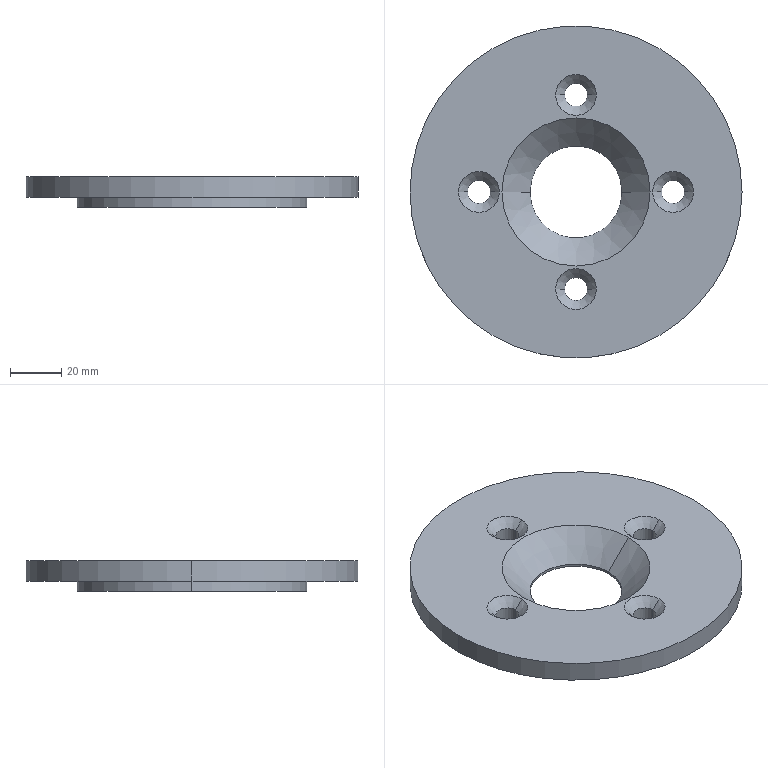Part | STEP file | PCA-130120 unmachined | 1 solid | 27 faces | box 130 x 130 x 12 mm | volume 107256 mm3 | cylinder 14 | cone 10 | plane 3 | commonest cylinder face diameters 9 x8 36 x2 90 x2 130 x2